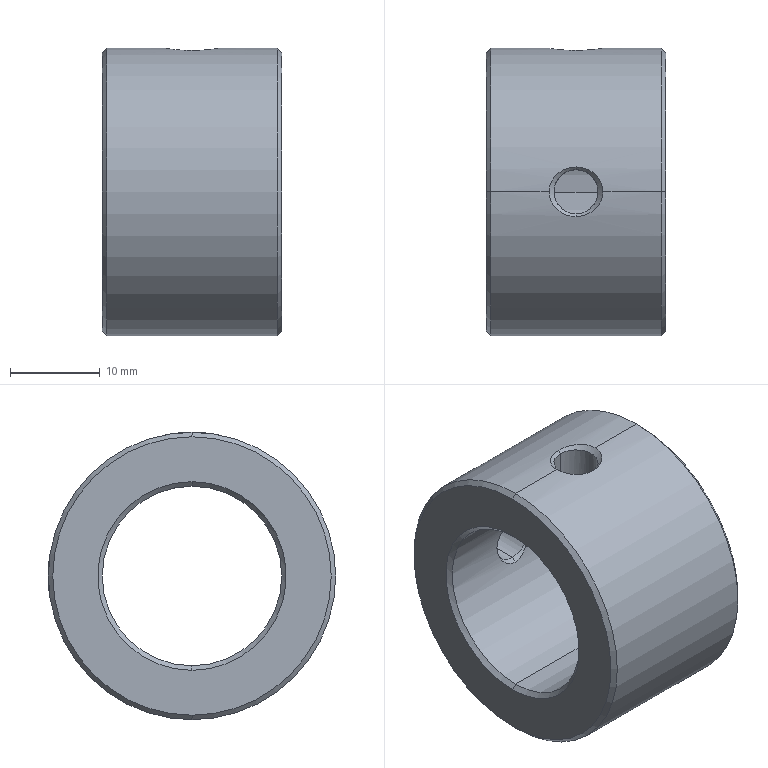Part | STEP file | SCCN20_20 | 1 solid | 28 faces | box 20 x 32 x 32 mm | volume 9528 mm3 | cone 18 | cylinder 8 | plane 2 | commonest cylinder face diameters 4.917 x4 20 x2 32 x2
STEP:
#1=CARTESIAN_POINT('',(0.,-2.458,15.459));
#2=VERTEX_POINT('',#1);
#3=CARTESIAN_POINT('',(0.,2.459,15.459));
#4=VERTEX_POINT('',#3);
#5=CARTESIAN_POINT('',(0.,0.,15.459));
#6=DIRECTION('',(0.,0.,-1.));
#7=DIRECTION('',(0.,1.,0.));
#8=AXIS2_PLACEMENT_3D('',#5,#6,#7);
#9=CIRCLE('',#8,2.459);
#10=EDGE_CURVE('',#2,#4,#9,.T.);
#11=ORIENTED_EDGE('',*,*,#10,.F.);
#12=CARTESIAN_POINT('',(0.,-2.458,10.));
#13=VERTEX_POINT('',#12);
#14=CARTESIAN_POINT('',(0.,-2.458,16.));
#15=DIRECTION('',(0.,0.,-1.));
#16=VECTOR('',#15,1000.);
#17=LINE('',#14,#16);
#18=EDGE_CURVE('',#2,#13,#17,.T.);
#19=ORIENTED_EDGE('',*,*,#18,.T.);
#20=CARTESIAN_POINT('',(-2.458,0.,10.));
#21=VERTEX_POINT('',#20);
#22=CARTESIAN_POINT('',(0.,0.,10.));
#23=DIRECTION('',(0.,0.,-1.));
#24=DIRECTION('',(0.,1.,0.));
#25=AXIS2_PLACEMENT_3D('',#22,#23,#24);
#26=CIRCLE('',#25,2.458);
#27=EDGE_CURVE('',#13,#21,#26,.T.);
#28=ORIENTED_EDGE('',*,*,#27,.T.);
#29=CARTESIAN_POINT('',(0.,2.459,10.));
#30=VERTEX_POINT('',#29);
#31=CARTESIAN_POINT('',(0.,0.,10.));
#32=DIRECTION('',(0.,0.,-1.));
#33=DIRECTION('',(0.,1.,0.));
#34=AXIS2_PLACEMENT_3D('',#31,#32,#33);
#35=CIRCLE('',#34,2.458);
#36=EDGE_CURVE('',#21,#30,#35,.T.);
#37=ORIENTED_EDGE('',*,*,#36,.T.);
#38=CARTESIAN_POINT('',(0.,2.459,16.));
#39=DIRECTION('',(0.,0.,-1.));
#40=VECTOR('',#39,1000.);
#41=LINE('',#38,#40);
#42=EDGE_CURVE('',#4,#30,#41,.T.);
#43=ORIENTED_EDGE('',*,*,#42,.F.);
#44=EDGE_LOOP('',(#11,#19,#28,#37,#43));
#45=FACE_OUTER_BOUND('',#44,.T.);
#46=CARTESIAN_POINT('',(0.,0.,16.));
#47=DIRECTION('',(0.,0.,-1.));
#48=DIRECTION('',(0.,1.,0.));
#49=AXIS2_PLACEMENT_3D('',#46,#47,#48);
#50=CYLINDRICAL_SURFACE('',#49,2.458);
#51=ADVANCED_FACE('',(#45),#50,.F.);
#52=ORIENTED_EDGE('',*,*,#10,.T.);
#53=CARTESIAN_POINT('',(0.,2.76,15.76));
#54=VERTEX_POINT('',#53);
#55=CARTESIAN_POINT('',(0.,3.,16.));
#56=DIRECTION('',(0.,0.7071,0.7071));
#57=VECTOR('',#56,1000.);
#58=LINE('',#55,#57);
#59=EDGE_CURVE('',#4,#54,#58,.T.);
#60=ORIENTED_EDGE('',*,*,#59,.T.);
#61=CARTESIAN_POINT('',(-3.,0.,16.));
#62=VERTEX_POINT('',#61);
#63=CARTESIAN_POINT('',(0.,2.76,15.76));
#64=CARTESIAN_POINT('',(-0.1883,2.76,15.76));
#65=CARTESIAN_POINT('',(-0.3793,2.743,15.763));
#66=CARTESIAN_POINT('',(-0.751,2.677,15.774));
#67=CARTESIAN_POINT('',(-0.9323,2.629,15.783));
#68=CARTESIAN_POINT('',(-1.285,2.499,15.804));
#69=CARTESIAN_POINT('',(-1.459,2.417,15.817));
#70=CARTESIAN_POINT('',(-1.782,2.225,15.845));
#71=CARTESIAN_POINT('',(-1.934,2.116,15.86));
#72=CARTESIAN_POINT('',(-2.216,1.867,15.891));
#73=CARTESIAN_POINT('',(-2.346,1.727,15.907));
#74=CARTESIAN_POINT('',(-2.573,1.428,15.937));
#75=CARTESIAN_POINT('',(-2.671,1.268,15.951));
#76=CARTESIAN_POINT('',(-2.832,0.9263,15.974));
#77=CARTESIAN_POINT('',(-2.895,0.7457,15.984));
#78=CARTESIAN_POINT('',(-2.978,0.3795,15.997));
#79=CARTESIAN_POINT('',(-3.,0.1901,16.));
#80=CARTESIAN_POINT('',(-3.,0.,16.));
#81=B_SPLINE_CURVE_WITH_KNOTS('',3,(#63,#64,#65,#66,#67,#68,#69,#70,#71,#72,#73,#74,#75,#76,#77,#78,#79,#80),.UNSPECIFIED.,.F.,.F.,(4,2,2,2,2,2,2,2,4),(0.01127,0.01184,0.0124,0.01297,0.01354,0.0141,0.01467,0.01523,0.0158),.UNSPECIFIED.);
#82=EDGE_CURVE('',#54,#62,#81,.T.);
#83=ORIENTED_EDGE('',*,*,#82,.T.);
#84=CARTESIAN_POINT('',(0.,-2.76,15.76));
#85=VERTEX_POINT('',#84);
#86=CARTESIAN_POINT('',(-3.,0.,16.));
#87=CARTESIAN_POINT('',(-3.,-0.1897,16.));
#88=CARTESIAN_POINT('',(-2.979,-0.3764,15.997));
#89=CARTESIAN_POINT('',(-2.896,-0.7442,15.984));
#90=CARTESIAN_POINT('',(-2.833,-0.9254,15.974));
#91=CARTESIAN_POINT('',(-2.672,-1.265,15.951));
#92=CARTESIAN_POINT('',(-2.574,-1.427,15.937));
#93=CARTESIAN_POINT('',(-2.345,-1.729,15.907));
#94=CARTESIAN_POINT('',(-2.216,-1.866,15.891));
#95=CARTESIAN_POINT('',(-1.932,-2.117,15.86));
#96=CARTESIAN_POINT('',(-1.779,-2.227,15.845));
#97=CARTESIAN_POINT('',(-1.456,-2.418,15.816));
#98=CARTESIAN_POINT('',(-1.283,-2.5,15.804));
#99=CARTESIAN_POINT('',(-0.9301,-2.629,15.783));
#100=CARTESIAN_POINT('',(-0.7491,-2.678,15.774));
#101=CARTESIAN_POINT('',(-0.3782,-2.744,15.763));
#102=CARTESIAN_POINT('',(-0.1877,-2.76,15.76));
#103=CARTESIAN_POINT('',(0.,-2.76,15.76));
#104=B_SPLINE_CURVE_WITH_KNOTS('',3,(#86,#87,#88,#89,#90,#91,#92,#93,#94,#95,#96,#97,#98,#99,#100,#101,#102,#103),.UNSPECIFIED.,.F.,.F.,(4,2,2,2,2,2,2,2,4),(0.0158,0.01637,0.01693,0.0175,0.01806,0.01862,0.01919,0.01975,0.02032),.UNSPECIFIED.);
#105=EDGE_CURVE('',#62,#85,#104,.T.);
#106=ORIENTED_EDGE('',*,*,#105,.T.);
#107=CARTESIAN_POINT('',(0.,-3.,16.));
#108=DIRECTION('',(0.,-0.7071,0.7071));
#109=VECTOR('',#108,1000.);
#110=LINE('',#107,#109);
#111=EDGE_CURVE('',#2,#85,#110,.T.);
#112=ORIENTED_EDGE('',*,*,#111,.F.);
#113=EDGE_LOOP('',(#52,#60,#83,#106,#112));
#114=FACE_OUTER_BOUND('',#113,.T.);
#115=CARTESIAN_POINT('',(0.,0.,16.));
#116=DIRECTION('',(0.,0.,1.));
#117=DIRECTION('',(0.,-1.,0.));
#118=AXIS2_PLACEMENT_3D('',#115,#116,#117);
#119=CONICAL_SURFACE('',#118,3.,0.7854);
#120=ADVANCED_FACE('',(#114),#119,.F.);
#121=CARTESIAN_POINT('',(2.458,0.,10.));
#122=VERTEX_POINT('',#121);
#123=CARTESIAN_POINT('',(0.,0.,10.));
#124=DIRECTION('',(0.,0.,-1.));
#125=DIRECTION('',(0.,1.,0.));
#126=AXIS2_PLACEMENT_3D('',#123,#124,#125);
#127=CIRCLE('',#126,2.458);
#128=EDGE_CURVE('',#30,#122,#127,.T.);
#129=ORIENTED_EDGE('',*,*,#128,.F.);
#130=CARTESIAN_POINT('',(0.,2.883,9.575));
#131=VERTEX_POINT('',#130);
#132=CARTESIAN_POINT('',(0.,2.459,10.));
#133=DIRECTION('',(0.,0.7071,-0.7071));
#134=VECTOR('',#133,1000.);
#135=LINE('',#132,#134);
#136=EDGE_CURVE('',#30,#131,#135,.T.);
#137=ORIENTED_EDGE('',*,*,#136,.T.);
#138=CARTESIAN_POINT('',(0.,2.883,9.575));
#139=CARTESIAN_POINT('',(0.1747,2.883,9.575));
#140=CARTESIAN_POINT('',(0.3527,2.86,9.583));
#141=CARTESIAN_POINT('',(0.691,2.77,9.609));
#142=CARTESIAN_POINT('',(0.855,2.704,9.628));
#143=CARTESIAN_POINT('',(1.316,2.454,9.696));
#144=CARTESIAN_POINT('',(1.582,2.219,9.755));
#145=CARTESIAN_POINT('',(1.905,1.812,9.836));
#146=CARTESIAN_POINT('',(2.001,1.664,9.862));
#147=CARTESIAN_POINT('',(2.165,1.357,9.909));
#148=CARTESIAN_POINT('',(2.234,1.198,9.929));
#149=CARTESIAN_POINT('',(2.346,0.867,9.964));
#150=CARTESIAN_POINT('',(2.388,0.6945,9.977));
#151=CARTESIAN_POINT('',(2.444,0.3492,9.995));
#152=CARTESIAN_POINT('',(2.459,0.1752,10.));
#153=CARTESIAN_POINT('',(2.458,0.,10.));
#154=B_SPLINE_CURVE_WITH_KNOTS('',3,(#138,#139,#140,#141,#142,#143,#144,#145,#146,#147,#148,#149,#150,#151,#152,#153),.UNSPECIFIED.,.F.,.F.,(4,2,2,2,2,2,2,4),(0.006307,0.00683,0.007353,0.008399,0.008922,0.009445,0.009968,0.01049),.UNSPECIFIED.);
#155=EDGE_CURVE('',#131,#122,#154,.T.);
#156=ORIENTED_EDGE('',*,*,#155,.T.);
#157=EDGE_LOOP('',(#129,#137,#156));
#158=FACE_OUTER_BOUND('',#157,.T.);
#159=CARTESIAN_POINT('',(0.,0.,10.));
#160=DIRECTION('',(0.,0.,-1.));
#161=DIRECTION('',(0.,1.,0.));
#162=AXIS2_PLACEMENT_3D('',#159,#160,#161);
#163=CONICAL_SURFACE('',#162,2.458,0.7854);
#164=ADVANCED_FACE('',(#158),#163,.F.);
#165=CARTESIAN_POINT('',(0.,15.459,2.458));
#166=VERTEX_POINT('',#165);
#167=CARTESIAN_POINT('',(0.,15.459,-2.459));
#168=VERTEX_POINT('',#167);
#169=CARTESIAN_POINT('',(0.,15.459,0.));
#170=DIRECTION('',(0.,-1.,0.));
#171=DIRECTION('',(0.,0.,-1.));
#172=AXIS2_PLACEMENT_3D('',#169,#170,#171);
#173=CIRCLE('',#172,2.458);
#174=EDGE_CURVE('',#166,#168,#173,.T.);
#175=ORIENTED_EDGE('',*,*,#174,.F.);
#176=CARTESIAN_POINT('',(0.,10.,2.458));
#177=VERTEX_POINT('',#176);
#178=CARTESIAN_POINT('',(0.,16.,2.458));
#179=DIRECTION('',(0.,-1.,0.));
#180=VECTOR('',#179,1000.);
#181=LINE('',#178,#180);
#182=EDGE_CURVE('',#166,#177,#181,.T.);
#183=ORIENTED_EDGE('',*,*,#182,.T.);
#184=CARTESIAN_POINT('',(-2.458,10.,0.));
#185=VERTEX_POINT('',#184);
#186=CARTESIAN_POINT('',(0.,10.,0.));
#187=DIRECTION('',(0.,-1.,0.));
#188=DIRECTION('',(0.,0.,-1.));
#189=AXIS2_PLACEMENT_3D('',#186,#187,#188);
#190=CIRCLE('',#189,2.458);
#191=EDGE_CURVE('',#177,#185,#190,.T.);
#192=ORIENTED_EDGE('',*,*,#191,.T.);
#193=CARTESIAN_POINT('',(0.,10.,-2.459));
#194=VERTEX_POINT('',#193);
#195=CARTESIAN_POINT('',(0.,10.,0.));
#196=DIRECTION('',(0.,-1.,0.));
#197=DIRECTION('',(0.,0.,-1.));
#198=AXIS2_PLACEMENT_3D('',#195,#196,#197);
#199=CIRCLE('',#198,2.458);
#200=EDGE_CURVE('',#185,#194,#199,.T.);
#201=ORIENTED_EDGE('',*,*,#200,.T.);
#202=CARTESIAN_POINT('',(0.,16.,-2.459));
#203=DIRECTION('',(0.,-1.,0.));
#204=VECTOR('',#203,1000.);
#205=LINE('',#202,#204);
#206=EDGE_CURVE('',#168,#194,#205,.T.);
#207=ORIENTED_EDGE('',*,*,#206,.F.);
#208=EDGE_LOOP('',(#175,#183,#192,#201,#207));
#209=FACE_OUTER_BOUND('',#208,.T.);
#210=CARTESIAN_POINT('',(0.,16.,0.));
#211=DIRECTION('',(0.,-1.,0.));
#212=DIRECTION('',(0.,0.,-1.));
#213=AXIS2_PLACEMENT_3D('',#210,#211,#212);
#214=CYLINDRICAL_SURFACE('',#213,2.458);
#215=ADVANCED_FACE('',(#209),#214,.F.);
#216=ORIENTED_EDGE('',*,*,#174,.T.);
#217=CARTESIAN_POINT('',(0.,15.76,-2.76));
#218=VERTEX_POINT('',#217);
#219=CARTESIAN_POINT('',(0.,16.,-3.));
#220=DIRECTION('',(0.,0.7071,-0.7071));
#221=VECTOR('',#220,1000.);
#222=LINE('',#219,#221);
#223=EDGE_CURVE('',#168,#218,#222,.T.);
#224=ORIENTED_EDGE('',*,*,#223,.T.);
#225=CARTESIAN_POINT('',(0.,15.76,2.76));
#226=VERTEX_POINT('',#225);
#227=CARTESIAN_POINT('',(0.,15.76,-2.76));
#228=CARTESIAN_POINT('',(-0.1888,15.76,-2.76));
#229=CARTESIAN_POINT('',(-0.3797,15.763,-2.743));
#230=CARTESIAN_POINT('',(-0.7498,15.774,-2.678));
#231=CARTESIAN_POINT('',(-0.9311,15.783,-2.629));
#232=CARTESIAN_POINT('',(-1.286,15.804,-2.499));
#233=CARTESIAN_POINT('',(-1.458,15.817,-2.417));
#234=CARTESIAN_POINT('',(-1.781,15.845,-2.226));
#235=CARTESIAN_POINT('',(-1.935,15.86,-2.115));
#236=CARTESIAN_POINT('',(-2.218,15.892,-1.864));
#237=CARTESIAN_POINT('',(-2.346,15.907,-1.727));
#238=CARTESIAN_POINT('',(-2.574,15.937,-1.427));
#239=CARTESIAN_POINT('',(-2.673,15.951,-1.263));
#240=CARTESIAN_POINT('',(-2.833,15.974,-0.9243));
#241=CARTESIAN_POINT('',(-2.895,15.984,-0.7473));
#242=CARTESIAN_POINT('',(-2.979,15.997,-0.3774));
#243=CARTESIAN_POINT('',(-3.,16.,-0.1885));
#244=CARTESIAN_POINT('',(-3.,16.,0.1871));
#245=CARTESIAN_POINT('',(-2.979,15.997,0.3778));
#246=CARTESIAN_POINT('',(-2.895,15.984,0.7461));
#247=CARTESIAN_POINT('',(-2.833,15.974,0.9237));
#248=CARTESIAN_POINT('',(-2.672,15.951,1.266));
#249=CARTESIAN_POINT('',(-2.573,15.937,1.428));
#250=CARTESIAN_POINT('',(-2.346,15.907,1.727));
#251=CARTESIAN_POINT('',(-2.216,15.891,1.867));
#252=CARTESIAN_POINT('',(-1.933,15.86,2.116));
#253=CARTESIAN_POINT('',(-1.781,15.845,2.226));
#254=CARTESIAN_POINT('',(-1.457,15.817,2.418));
#255=CARTESIAN_POINT('',(-1.284,15.804,2.499));
#256=CARTESIAN_POINT('',(-0.9317,15.783,2.629));
#257=CARTESIAN_POINT('',(-0.7503,15.774,2.678));
#258=CARTESIAN_POINT('',(-0.377,15.763,2.744));
#259=CARTESIAN_POINT('',(-0.1877,15.76,2.76));
#260=CARTESIAN_POINT('',(0.,15.76,2.76));
#261=B_SPLINE_CURVE_WITH_KNOTS('',3,(#227,#228,#229,#230,#231,#232,#233,#234,#235,#236,#237,#238,#239,#240,#241,#242,#243,#244,#245,#246,#247,#248,#249,#250,#251,#252,#253,#254,#255,#256,#257,#258,#259,#260),.UNSPECIFIED.,.F.,.F.,(4,2,2,2,2,2,2,2,2,2,2,2,2,2,2,2,4),(0.01587,0.01644,0.017,0.01757,0.01813,0.0187,0.01926,0.01983,0.02039,0.02096,0.02152,0.02209,0.02265,0.02322,0.02378,0.02435,0.02491),.UNSPECIFIED.);
#262=EDGE_CURVE('',#218,#226,#261,.T.);
#263=ORIENTED_EDGE('',*,*,#262,.T.);
#264=CARTESIAN_POINT('',(0.,16.,3.));
#265=DIRECTION('',(0.,0.7071,0.7071));
#266=VECTOR('',#265,1000.);
#267=LINE('',#264,#266);
#268=EDGE_CURVE('',#166,#226,#267,.T.);
#269=ORIENTED_EDGE('',*,*,#268,.F.);
#270=EDGE_LOOP('',(#216,#224,#263,#269));
#271=FACE_OUTER_BOUND('',#270,.T.);
#272=CARTESIAN_POINT('',(0.,16.,0.));
#273=DIRECTION('',(0.,1.,0.));
#274=DIRECTION('',(0.,0.,1.));
#275=AXIS2_PLACEMENT_3D('',#272,#273,#274);
#276=CONICAL_SURFACE('',#275,3.,0.7854);
#277=ADVANCED_FACE('',(#271),#276,.F.);
#278=CARTESIAN_POINT('',(2.458,10.,0.));
#279=VERTEX_POINT('',#278);
#280=CARTESIAN_POINT('',(0.,10.,0.));
#281=DIRECTION('',(0.,-1.,0.));
#282=DIRECTION('',(0.,0.,-1.));
#283=AXIS2_PLACEMENT_3D('',#280,#281,#282);
#284=CIRCLE('',#283,2.458);
#285=EDGE_CURVE('',#194,#279,#284,.T.);
#286=ORIENTED_EDGE('',*,*,#285,.F.);
#287=CARTESIAN_POINT('',(0.,9.575,-2.883));
#288=VERTEX_POINT('',#287);
#289=CARTESIAN_POINT('',(0.,10.,-2.459));
#290=DIRECTION('',(0.,-0.7071,-0.7071));
#291=VECTOR('',#290,1000.);
#292=LINE('',#289,#291);
#293=EDGE_CURVE('',#194,#288,#292,.T.);
#294=ORIENTED_EDGE('',*,*,#293,.T.);
#295=CARTESIAN_POINT('',(0.,9.575,-2.883));
#296=CARTESIAN_POINT('',(0.1752,9.575,-2.883));
#297=CARTESIAN_POINT('',(0.3529,9.583,-2.86));
#298=CARTESIAN_POINT('',(0.6907,9.609,-2.77));
#299=CARTESIAN_POINT('',(0.8557,9.628,-2.704));
#300=CARTESIAN_POINT('',(1.315,9.696,-2.454));
#301=CARTESIAN_POINT('',(1.582,9.754,-2.22));
#302=CARTESIAN_POINT('',(1.905,9.836,-1.811));
#303=CARTESIAN_POINT('',(2.001,9.862,-1.664));
#304=CARTESIAN_POINT('',(2.165,9.909,-1.358));
#305=CARTESIAN_POINT('',(2.234,9.929,-1.198));
#306=CARTESIAN_POINT('',(2.346,9.964,-0.8661));
#307=CARTESIAN_POINT('',(2.388,9.977,-0.6947));
#308=CARTESIAN_POINT('',(2.444,9.995,-0.3503));
#309=CARTESIAN_POINT('',(2.459,10.,-0.1762));
#310=CARTESIAN_POINT('',(2.458,10.,0.));
#311=B_SPLINE_CURVE_WITH_KNOTS('',3,(#295,#296,#297,#298,#299,#300,#301,#302,#303,#304,#305,#306,#307,#308,#309,#310),.UNSPECIFIED.,.F.,.F.,(4,2,2,2,2,2,2,4),(0.002095,0.00262,0.003146,0.004197,0.004723,0.005249,0.005774,0.0063),.UNSPECIFIED.);
#312=EDGE_CURVE('',#288,#279,#311,.T.);
#313=ORIENTED_EDGE('',*,*,#312,.T.);
#314=EDGE_LOOP('',(#286,#294,#313));
#315=FACE_OUTER_BOUND('',#314,.T.);
#316=CARTESIAN_POINT('',(0.,10.,0.));
#317=DIRECTION('',(0.,-1.,0.));
#318=DIRECTION('',(0.,0.,-1.));
#319=AXIS2_PLACEMENT_3D('',#316,#317,#318);
#320=CONICAL_SURFACE('',#319,2.458,0.7854);
#321=ADVANCED_FACE('',(#315),#320,.F.);
#322=CARTESIAN_POINT('',(-10.,0.,15.5));
#323=VERTEX_POINT('',#322);
#324=CARTESIAN_POINT('',(-10.,0.,-15.5));
#325=VERTEX_POINT('',#324);
#326=CARTESIAN_POINT('',(-10.,0.,0.));
#327=DIRECTION('',(-1.,0.,0.));
#328=DIRECTION('',(0.,0.,1.));
#329=AXIS2_PLACEMENT_3D('',#326,#327,#328);
#330=CIRCLE('',#329,15.5);
#331=EDGE_CURVE('',#323,#325,#330,.T.);
#332=ORIENTED_EDGE('',*,*,#331,.F.);
#333=CARTESIAN_POINT('',(-9.5,0.,16.));
#334=VERTEX_POINT('',#333);
#335=CARTESIAN_POINT('',(-9.5,0.,16.));
#336=DIRECTION('',(0.7071,0.,0.7071));
#337=VECTOR('',#336,1000.);
#338=LINE('',#335,#337);
#339=EDGE_CURVE('',#323,#334,#338,.T.);
#340=ORIENTED_EDGE('',*,*,#339,.T.);
#341=CARTESIAN_POINT('',(-9.5,0.,-16.));
#342=VERTEX_POINT('',#341);
#343=CARTESIAN_POINT('',(-9.5,0.,0.));
#344=DIRECTION('',(-1.,0.,0.));
#345=DIRECTION('',(0.,0.,1.));
#346=AXIS2_PLACEMENT_3D('',#343,#344,#345);
#347=CIRCLE('',#346,16.);
#348=EDGE_CURVE('',#334,#342,#347,.T.);
#349=ORIENTED_EDGE('',*,*,#348,.T.);
#350=CARTESIAN_POINT('',(-9.5,0.,-16.));
#351=DIRECTION('',(0.7071,0.,-0.7071));
#352=VECTOR('',#351,1000.);
#353=LINE('',#350,#352);
#354=EDGE_CURVE('',#325,#342,#353,.T.);
#355=ORIENTED_EDGE('',*,*,#354,.F.);
#356=EDGE_LOOP('',(#332,#340,#349,#355));
#357=FACE_OUTER_BOUND('',#356,.T.);
#358=CARTESIAN_POINT('',(-9.5,0.,0.));
#359=DIRECTION('',(1.,0.,0.));
#360=DIRECTION('',(0.,0.,-1.));
#361=AXIS2_PLACEMENT_3D('',#358,#359,#360);
#362=CONICAL_SURFACE('',#361,16.,0.7854);
#363=ADVANCED_FACE('',(#357),#362,.T.);
#364=CARTESIAN_POINT('',(10.,0.,15.5));
#365=VERTEX_POINT('',#364);
#366=CARTESIAN_POINT('',(10.,0.,-15.5));
#367=VERTEX_POINT('',#366);
#368=CARTESIAN_POINT('',(10.,0.,0.));
#369=DIRECTION('',(-1.,0.,0.));
#370=DIRECTION('',(0.,0.,1.));
#371=AXIS2_PLACEMENT_3D('',#368,#369,#370);
#372=CIRCLE('',#371,15.5);
#373=EDGE_CURVE('',#365,#367,#372,.T.);
#374=ORIENTED_EDGE('',*,*,#373,.T.);
#375=CARTESIAN_POINT('',(9.5,0.,-16.));
#376=VERTEX_POINT('',#375);
#377=CARTESIAN_POINT('',(10.,0.,-15.5));
#378=DIRECTION('',(-0.7071,0.,-0.7071));
#379=VECTOR('',#378,1000.);
#380=LINE('',#377,#379);
#381=EDGE_CURVE('',#367,#376,#380,.T.);
#382=ORIENTED_EDGE('',*,*,#381,.T.);
#383=CARTESIAN_POINT('',(9.5,0.,16.));
#384=VERTEX_POINT('',#383);
#385=CARTESIAN_POINT('',(9.5,0.,0.));
#386=DIRECTION('',(-1.,0.,0.));
#387=DIRECTION('',(0.,0.,1.));
#388=AXIS2_PLACEMENT_3D('',#385,#386,#387);
#389=CIRCLE('',#388,16.);
#390=EDGE_CURVE('',#384,#376,#389,.T.);
#391=ORIENTED_EDGE('',*,*,#390,.F.);
#392=CARTESIAN_POINT('',(10.,0.,15.5));
#393=DIRECTION('',(-0.7071,0.,0.7071));
#394=VECTOR('',#393,1000.);
#395=LINE('',#392,#394);
#396=EDGE_CURVE('',#365,#384,#395,.T.);
#397=ORIENTED_EDGE('',*,*,#396,.F.);
#398=EDGE_LOOP('',(#374,#382,#391,#397));
#399=FACE_OUTER_BOUND('',#398,.T.);
#400=CARTESIAN_POINT('',(10.,0.,0.));
#401=DIRECTION('',(-1.,0.,0.));
#402=DIRECTION('',(0.,0.,1.));
#403=AXIS2_PLACEMENT_3D('',#400,#401,#402);
#404=CONICAL_SURFACE('',#403,15.5,0.7854);
#405=ADVANCED_FACE('',(#399),#404,.T.);
#406=CARTESIAN_POINT('',(9.5,0.,-10.));
#407=VERTEX_POINT('',#406);
#408=CARTESIAN_POINT('',(9.5,0.,10.));
#409=VERTEX_POINT('',#408);
#410=CARTESIAN_POINT('',(9.5,0.,0.));
#411=DIRECTION('',(-1.,0.,0.));
#412=DIRECTION('',(0.,0.,1.));
#413=AXIS2_PLACEMENT_3D('',#410,#411,#412);
#414=CIRCLE('',#413,10.);
#415=EDGE_CURVE('',#407,#409,#414,.T.);
#416=ORIENTED_EDGE('',*,*,#415,.T.);
#417=CARTESIAN_POINT('',(10.,0.,10.5));
#418=VERTEX_POINT('',#417);
#419=CARTESIAN_POINT('',(9.5,0.,10.));
#420=DIRECTION('',(0.7071,0.,0.7071));
#421=VECTOR('',#420,1000.);
#422=LINE('',#419,#421);
#423=EDGE_CURVE('',#409,#418,#422,.T.);
#424=ORIENTED_EDGE('',*,*,#423,.T.);
#425=CARTESIAN_POINT('',(10.,0.,-10.5));
#426=VERTEX_POINT('',#425);
#427=CARTESIAN_POINT('',(10.,0.,0.));
#428=DIRECTION('',(-1.,0.,0.));
#429=DIRECTION('',(0.,0.,1.));
#430=AXIS2_PLACEMENT_3D('',#427,#428,#429);
#431=CIRCLE('',#430,10.5);
#432=EDGE_CURVE('',#426,#418,#431,.T.);
#433=ORIENTED_EDGE('',*,*,#432,.F.);
#434=CARTESIAN_POINT('',(9.5,0.,-10.));
#435=DIRECTION('',(0.7071,0.,-0.7071));
#436=VECTOR('',#435,1000.);
#437=LINE('',#434,#436);
#438=EDGE_CURVE('',#407,#426,#437,.T.);
#439=ORIENTED_EDGE('',*,*,#438,.F.);
#440=EDGE_LOOP('',(#416,#424,#433,#439));
#441=FACE_OUTER_BOUND('',#440,.T.);
#442=CARTESIAN_POINT('',(9.5,0.,0.));
#443=DIRECTION('',(1.,0.,0.));
#444=DIRECTION('',(0.,0.,-1.));
#445=AXIS2_PLACEMENT_3D('',#442,#443,#444);
#446=CONICAL_SURFACE('',#445,10.,0.7854);
#447=ADVANCED_FACE('',(#441),#446,.F.);
#448=CARTESIAN_POINT('',(-9.5,0.,-10.));
#449=VERTEX_POINT('',#448);
#450=CARTESIAN_POINT('',(-9.5,0.,10.));
#451=VERTEX_POINT('',#450);
#452=CARTESIAN_POINT('',(-9.5,0.,0.));
#453=DIRECTION('',(-1.,0.,0.));
#454=DIRECTION('',(0.,0.,1.));
#455=AXIS2_PLACEMENT_3D('',#452,#453,#454);
#456=CIRCLE('',#455,10.);
#457=EDGE_CURVE('',#449,#451,#456,.T.);
#458=ORIENTED_EDGE('',*,*,#457,.F.);
#459=CARTESIAN_POINT('',(-10.,0.,-10.5));
#460=VERTEX_POINT('',#459);
#461=CARTESIAN_POINT('',(-10.,0.,-10.5));
#462=DIRECTION('',(-0.7071,0.,-0.7071));
#463=VECTOR('',#462,1000.);
#464=LINE('',#461,#463);
#465=EDGE_CURVE('',#449,#460,#464,.T.);
#466=ORIENTED_EDGE('',*,*,#465,.T.);
#467=CARTESIAN_POINT('',(-10.,0.,10.5));
#468=VERTEX_POINT('',#467);
#469=CARTESIAN_POINT('',(-10.,0.,0.));
#470=DIRECTION('',(-1.,0.,0.));
#471=DIRECTION('',(0.,0.,1.));
#472=AXIS2_PLACEMENT_3D('',#469,#470,#471);
#473=CIRCLE('',#472,10.5);
#474=EDGE_CURVE('',#460,#468,#473,.T.);
#475=ORIENTED_EDGE('',*,*,#474,.T.);
#476=CARTESIAN_POINT('',(-10.,0.,10.5));
#477=DIRECTION('',(-0.7071,0.,0.7071));
#478=VECTOR('',#477,1000.);
#479=LINE('',#476,#478);
#480=EDGE_CURVE('',#451,#468,#479,.T.);
#481=ORIENTED_EDGE('',*,*,#480,.F.);
#482=EDGE_LOOP('',(#458,#466,#475,#481));
#483=FACE_OUTER_BOUND('',#482,.T.);
#484=CARTESIAN_POINT('',(-10.,0.,0.));
#485=DIRECTION('',(-1.,0.,0.));
#486=DIRECTION('',(0.,0.,1.));
#487=AXIS2_PLACEMENT_3D('',#484,#485,#486);
#488=CONICAL_SURFACE('',#487,10.5,0.7854);
#489=ADVANCED_FACE('',(#483),#488,.F.);
#490=CARTESIAN_POINT('',(0.,15.76,2.76));
#491=CARTESIAN_POINT('',(0.3757,15.76,2.76));
#492=CARTESIAN_POINT('',(0.7561,15.772,2.693));
#493=CARTESIAN_POINT('',(1.46,15.814,2.435));
#494=CARTESIAN_POINT('',(1.793,15.844,2.24));
#495=CARTESIAN_POINT('',(2.213,15.891,1.869));
#496=CARTESIAN_POINT('',(2.344,15.907,1.73));
#497=CARTESIAN_POINT('',(2.572,15.937,1.43));
#498=CARTESIAN_POINT('',(2.67,15.95,1.27));
#499=CARTESIAN_POINT('',(2.831,15.974,0.9309));
#500=CARTESIAN_POINT('',(2.894,15.984,0.7492));
#501=CARTESIAN_POINT('',(2.978,15.996,0.382));
#502=CARTESIAN_POINT('',(3.,16.,0.1953));
#503=CARTESIAN_POINT('',(3.,16.,-0.1841));
#504=CARTESIAN_POINT('',(2.979,15.997,-0.374));
#505=CARTESIAN_POINT('',(2.896,15.984,-0.7411));
#506=CARTESIAN_POINT('',(2.834,15.974,-0.9225));
#507=CARTESIAN_POINT('',(2.673,15.951,-1.264));
#508=CARTESIAN_POINT('',(2.575,15.937,-1.425));
#509=CARTESIAN_POINT('',(2.347,15.907,-1.726));
#510=CARTESIAN_POINT('',(2.217,15.891,-1.865));
#511=CARTESIAN_POINT('',(1.936,15.86,-2.114));
#512=CARTESIAN_POINT('',(1.781,15.845,-2.226));
#513=CARTESIAN_POINT('',(1.456,15.816,-2.418));
#514=CARTESIAN_POINT('',(1.286,15.804,-2.499));
#515=CARTESIAN_POINT('',(0.9327,15.783,-2.629));
#516=CARTESIAN_POINT('',(0.7475,15.774,-2.678));
#517=CARTESIAN_POINT('',(0.3762,15.763,-2.744));
#518=CARTESIAN_POINT('',(0.1889,15.76,-2.76));
#519=CARTESIAN_POINT('',(0.,15.76,-2.76));
#520=B_SPLINE_CURVE_WITH_KNOTS('',3,(#490,#491,#492,#493,#494,#495,#496,#497,#498,#499,#500,#501,#502,#503,#504,#505,#506,#507,#508,#509,#510,#511,#512,#513,#514,#515,#516,#517,#518,#519),.UNSPECIFIED.,.F.,.F.,(4,2,2,2,2,2,2,2,2,2,2,2,2,2,4),(0.006826,0.007957,0.009088,0.009653,0.01022,0.01078,0.01135,0.01191,0.01248,0.01305,0.01361,0.01418,0.01474,0.01531,0.01587),.UNSPECIFIED.);
#521=EDGE_CURVE('',#226,#218,#520,.T.);
#522=ORIENTED_EDGE('',*,*,#521,.F.);
#523=ORIENTED_EDGE('',*,*,#262,.F.);
#524=EDGE_LOOP('',(#522,#523));
#525=FACE_BOUND('',#524,.T.);
#526=ORIENTED_EDGE('',*,*,#390,.T.);
#527=CARTESIAN_POINT('',(5.,0.,-16.));
#528=DIRECTION('',(-1.,0.,0.));
#529=VECTOR('',#528,1000.);
#530=LINE('',#527,#529);
#531=EDGE_CURVE('',#376,#342,#530,.T.);
#532=ORIENTED_EDGE('',*,*,#531,.T.);
#533=ORIENTED_EDGE('',*,*,#348,.F.);
#534=CARTESIAN_POINT('',(5.,0.,16.));
#535=DIRECTION('',(-1.,0.,0.));
#536=VECTOR('',#535,1000.);
#537=LINE('',#534,#536);
#538=EDGE_CURVE('',#62,#334,#537,.T.);
#539=ORIENTED_EDGE('',*,*,#538,.F.);
#540=ORIENTED_EDGE('',*,*,#82,.F.);
#541=CARTESIAN_POINT('',(3.,0.,16.));
#542=VERTEX_POINT('',#541);
#543=CARTESIAN_POINT('',(3.,0.,16.));
#544=CARTESIAN_POINT('',(3.,0.1885,16.));
#545=CARTESIAN_POINT('',(2.978,0.3795,15.997));
#546=CARTESIAN_POINT('',(2.895,0.7462,15.984));
#547=CARTESIAN_POINT('',(2.833,0.9257,15.974));
#548=CARTESIAN_POINT('',(2.671,1.268,15.951));
#549=CARTESIAN_POINT('',(2.573,1.428,15.937));
#550=CARTESIAN_POINT('',(2.345,1.728,15.907));
#551=CARTESIAN_POINT('',(2.215,1.868,15.891));
#552=CARTESIAN_POINT('',(1.792,2.24,15.844));
#553=CARTESIAN_POINT('',(1.46,2.435,15.814));
#554=CARTESIAN_POINT('',(0.9316,2.629,15.783));
#555=CARTESIAN_POINT('',(0.7476,2.678,15.774));
#556=CARTESIAN_POINT('',(0.3751,2.744,15.763));
#557=CARTESIAN_POINT('',(0.188,2.76,15.76));
#558=CARTESIAN_POINT('',(0.,2.76,15.76));
#559=B_SPLINE_CURVE_WITH_KNOTS('',3,(#543,#544,#545,#546,#547,#548,#549,#550,#551,#552,#553,#554,#555,#556,#557,#558),.UNSPECIFIED.,.F.,.F.,(4,2,2,2,2,2,2,4),(0.006751,0.007316,0.007881,0.008446,0.009012,0.01014,0.01071,0.01127),.UNSPECIFIED.);
#560=EDGE_CURVE('',#542,#54,#559,.T.);
#561=ORIENTED_EDGE('',*,*,#560,.F.);
#562=CARTESIAN_POINT('',(5.,0.,16.));
#563=DIRECTION('',(-1.,0.,0.));
#564=VECTOR('',#563,1000.);
#565=LINE('',#562,#564);
#566=EDGE_CURVE('',#384,#542,#565,.T.);
#567=ORIENTED_EDGE('',*,*,#566,.F.);
#568=EDGE_LOOP('',(#526,#532,#533,#539,#540,#561,#567));
#569=FACE_OUTER_BOUND('',#568,.T.);
#570=CARTESIAN_POINT('',(5.,0.,0.));
#571=DIRECTION('',(-1.,0.,0.));
#572=DIRECTION('',(0.,0.,1.));
#573=AXIS2_PLACEMENT_3D('',#570,#571,#572);
#574=CYLINDRICAL_SURFACE('',#573,16.);
#575=ADVANCED_FACE('',(#525,#569),#574,.T.);
#576=ORIENTED_EDGE('',*,*,#415,.F.);
#577=CARTESIAN_POINT('',(5.,0.,-10.));
#578=DIRECTION('',(-1.,0.,0.));
#579=VECTOR('',#578,1000.);
#580=LINE('',#577,#579);
#581=EDGE_CURVE('',#407,#449,#580,.T.);
#582=ORIENTED_EDGE('',*,*,#581,.T.);
#583=ORIENTED_EDGE('',*,*,#457,.T.);
#584=CARTESIAN_POINT('',(5.,0.,10.));
#585=DIRECTION('',(-1.,0.,0.));
#586=VECTOR('',#585,1000.);
#587=LINE('',#584,#586);
#588=EDGE_CURVE('',#21,#451,#587,.T.);
#589=ORIENTED_EDGE('',*,*,#588,.F.);
#590=CARTESIAN_POINT('',(2.458,0.,10.));
#591=CARTESIAN_POINT('',(2.459,-0.1753,10.));
#592=CARTESIAN_POINT('',(2.444,-0.353,9.995));
#593=CARTESIAN_POINT('',(2.388,-0.6983,9.977));
#594=CARTESIAN_POINT('',(2.346,-0.8672,9.964));
#595=CARTESIAN_POINT('',(2.234,-1.198,9.929));
#596=CARTESIAN_POINT('',(2.164,-1.361,9.908));
#597=CARTESIAN_POINT('',(2.,-1.666,9.861));
#598=CARTESIAN_POINT('',(1.905,-1.811,9.836));
#599=CARTESIAN_POINT('',(1.69,-2.082,9.782));
#600=CARTESIAN_POINT('',(1.569,-2.21,9.753));
#601=CARTESIAN_POINT('',(1.306,-2.436,9.699));
#602=CARTESIAN_POINT('',(1.165,-2.536,9.674));
#603=CARTESIAN_POINT('',(0.8556,-2.704,9.628));
#604=CARTESIAN_POINT('',(0.6932,-2.769,9.609));
#605=CARTESIAN_POINT('',(0.3544,-2.859,9.583));
#606=CARTESIAN_POINT('',(0.1765,-2.883,9.575));
#607=CARTESIAN_POINT('',(-0.1734,-2.883,9.575));
#608=CARTESIAN_POINT('',(-0.3506,-2.86,9.582));
#609=CARTESIAN_POINT('',(-0.6906,-2.77,9.609));
#610=CARTESIAN_POINT('',(-0.8532,-2.705,9.628));
#611=CARTESIAN_POINT('',(-1.163,-2.537,9.673));
#612=CARTESIAN_POINT('',(-1.305,-2.437,9.699));
#613=CARTESIAN_POINT('',(-1.569,-2.21,9.753));
#614=CARTESIAN_POINT('',(-1.691,-2.082,9.782));
#615=CARTESIAN_POINT('',(-2.015,-1.671,9.863));
#616=CARTESIAN_POINT('',(-2.178,-1.364,9.912));
#617=CARTESIAN_POINT('',(-2.346,-0.8651,9.964));
#618=CARTESIAN_POINT('',(-2.388,-0.6959,9.977));
#619=CARTESIAN_POINT('',(-2.444,-0.352,9.995));
#620=CARTESIAN_POINT('',(-2.459,-0.1762,10.));
#621=CARTESIAN_POINT('',(-2.458,0.,10.));
#622=B_SPLINE_CURVE_WITH_KNOTS('',3,(#590,#591,#592,#593,#594,#595,#596,#597,#598,#599,#600,#601,#602,#603,#604,#605,#606,#607,#608,#609,#610,#611,#612,#613,#614,#615,#616,#617,#618,#619,#620,#621),.UNSPECIFIED.,.F.,.F.,(4,2,2,2,2,2,2,2,2,2,2,2,2,2,2,4),(0.01049,0.01101,0.01154,0.01206,0.01258,0.01311,0.01363,0.01415,0.01468,0.0152,0.01572,0.01625,0.01677,0.01782,0.01834,0.01886),.UNSPECIFIED.);
#623=EDGE_CURVE('',#122,#21,#622,.T.);
#624=ORIENTED_EDGE('',*,*,#623,.F.);
#625=CARTESIAN_POINT('',(5.,0.,10.));
#626=DIRECTION('',(-1.,0.,0.));
#627=VECTOR('',#626,1000.);
#628=LINE('',#625,#627);
#629=EDGE_CURVE('',#409,#122,#628,.T.);
#630=ORIENTED_EDGE('',*,*,#629,.F.);
#631=EDGE_LOOP('',(#576,#582,#583,#589,#624,#630));
#632=FACE_OUTER_BOUND('',#631,.T.);
#633=CARTESIAN_POINT('',(5.,0.,0.));
#634=DIRECTION('',(-1.,0.,0.));
#635=DIRECTION('',(0.,0.,1.));
#636=AXIS2_PLACEMENT_3D('',#633,#634,#635);
#637=CYLINDRICAL_SURFACE('',#636,10.);
#638=ADVANCED_FACE('',(#632),#637,.F.);
#639=ORIENTED_EDGE('',*,*,#581,.F.);
#640=CARTESIAN_POINT('',(9.5,0.,0.));
#641=DIRECTION('',(-1.,0.,0.));
#642=DIRECTION('',(0.,0.,1.));
#643=AXIS2_PLACEMENT_3D('',#640,#641,#642);
#644=CIRCLE('',#643,10.);
#645=EDGE_CURVE('',#409,#407,#644,.T.);
#646=ORIENTED_EDGE('',*,*,#645,.F.);
#647=ORIENTED_EDGE('',*,*,#629,.T.);
#648=ORIENTED_EDGE('',*,*,#155,.F.);
#649=CARTESIAN_POINT('',(-2.458,0.,10.));
#650=CARTESIAN_POINT('',(-2.459,0.1767,10.));
#651=CARTESIAN_POINT('',(-2.444,0.3512,9.995));
#652=CARTESIAN_POINT('',(-2.388,0.696,9.977));
#653=CARTESIAN_POINT('',(-2.346,0.8674,9.964));
#654=CARTESIAN_POINT('',(-2.233,1.201,9.929));
#655=CARTESIAN_POINT('',(-2.164,1.36,9.908));
#656=CARTESIAN_POINT('',(-2.,1.665,9.862));
#657=CARTESIAN_POINT('',(-1.904,1.812,9.835));
#658=CARTESIAN_POINT('',(-1.688,2.086,9.781));
#659=CARTESIAN_POINT('',(-1.569,2.211,9.753));
#660=CARTESIAN_POINT('',(-1.307,2.436,9.7));
#661=CARTESIAN_POINT('',(-1.163,2.537,9.673));
#662=CARTESIAN_POINT('',(-0.855,2.704,9.628));
#663=CARTESIAN_POINT('',(-0.6931,2.77,9.609));
#664=CARTESIAN_POINT('',(-0.3517,2.86,9.582));
#665=CARTESIAN_POINT('',(-0.1754,2.883,9.575));
#666=CARTESIAN_POINT('',(0.,2.883,9.575));
#667=B_SPLINE_CURVE_WITH_KNOTS('',3,(#649,#650,#651,#652,#653,#654,#655,#656,#657,#658,#659,#660,#661,#662,#663,#664,#665,#666),.UNSPECIFIED.,.F.,.F.,(4,2,2,2,2,2,2,2,4),(0.002109,0.002634,0.003158,0.003683,0.004208,0.004733,0.005258,0.005782,0.006307),.UNSPECIFIED.);
#668=EDGE_CURVE('',#21,#131,#667,.T.);
#669=ORIENTED_EDGE('',*,*,#668,.F.);
#670=ORIENTED_EDGE('',*,*,#588,.T.);
#671=CARTESIAN_POINT('',(-9.5,0.,0.));
#672=DIRECTION('',(-1.,0.,0.));
#673=DIRECTION('',(0.,0.,1.));
#674=AXIS2_PLACEMENT_3D('',#671,#672,#673);
#675=CIRCLE('',#674,10.);
#676=EDGE_CURVE('',#451,#449,#675,.T.);
#677=ORIENTED_EDGE('',*,*,#676,.T.);
#678=EDGE_LOOP('',(#639,#646,#647,#648,#669,#670,#677));
#679=FACE_OUTER_BOUND('',#678,.T.);
#680=CARTESIAN_POINT('',(2.458,10.,0.));
#681=CARTESIAN_POINT('',(2.459,10.,0.1762));
#682=CARTESIAN_POINT('',(2.444,9.995,0.3525));
#683=CARTESIAN_POINT('',(2.388,9.977,0.6966));
#684=CARTESIAN_POINT('',(2.346,9.964,0.8658));
#685=CARTESIAN_POINT('',(2.234,9.929,1.198));
#686=CARTESIAN_POINT('',(2.164,9.908,1.359));
#687=CARTESIAN_POINT('',(2.001,9.862,1.664));
#688=CARTESIAN_POINT('',(1.907,9.836,1.809));
#689=CARTESIAN_POINT('',(1.691,9.782,2.082));
#690=CARTESIAN_POINT('',(1.57,9.754,2.209));
#691=CARTESIAN_POINT('',(1.31,9.7,2.433));
#692=CARTESIAN_POINT('',(1.169,9.674,2.533));
#693=CARTESIAN_POINT('',(0.8617,9.629,2.701));
#694=CARTESIAN_POINT('',(0.6984,9.61,2.768));
#695=CARTESIAN_POINT('',(0.3601,9.583,2.858));
#696=CARTESIAN_POINT('',(0.182,9.576,2.883));
#697=CARTESIAN_POINT('',(-0.1682,9.575,2.884));
#698=CARTESIAN_POINT('',(-0.3451,9.582,2.861));
#699=CARTESIAN_POINT('',(-0.6858,9.608,2.772));
#700=CARTESIAN_POINT('',(-0.8481,9.627,2.707));
#701=CARTESIAN_POINT('',(-1.158,9.672,2.54));
#702=CARTESIAN_POINT('',(-1.301,9.698,2.44));
#703=CARTESIAN_POINT('',(-1.566,9.753,2.214));
#704=CARTESIAN_POINT('',(-1.687,9.781,2.086));
#705=CARTESIAN_POINT('',(-2.011,9.862,1.678));
#706=CARTESIAN_POINT('',(-2.178,9.912,1.364));
#707=CARTESIAN_POINT('',(-2.345,9.964,0.8689));
#708=CARTESIAN_POINT('',(-2.388,9.977,0.6975));
#709=CARTESIAN_POINT('',(-2.445,9.995,0.3494));
#710=CARTESIAN_POINT('',(-2.459,10.,0.1749));
#711=CARTESIAN_POINT('',(-2.458,10.,0.));
#712=B_SPLINE_CURVE_WITH_KNOTS('',3,(#680,#681,#682,#683,#684,#685,#686,#687,#688,#689,#690,#691,#692,#693,#694,#695,#696,#697,#698,#699,#700,#701,#702,#703,#704,#705,#706,#707,#708,#709,#710,#711),.UNSPECIFIED.,.F.,.F.,(4,2,2,2,2,2,2,2,2,2,2,2,2,2,2,4),(0.0063,0.006826,0.007351,0.007877,0.008403,0.008928,0.009454,0.00998,0.01051,0.01103,0.01156,0.01208,0.01261,0.01366,0.01418,0.01471),.UNSPECIFIED.);
#713=EDGE_CURVE('',#279,#185,#712,.T.);
#714=ORIENTED_EDGE('',*,*,#713,.F.);
#715=ORIENTED_EDGE('',*,*,#312,.F.);
#716=CARTESIAN_POINT('',(-2.458,10.,0.));
#717=CARTESIAN_POINT('',(-2.459,10.,-0.1749));
#718=CARTESIAN_POINT('',(-2.444,9.995,-0.3515));
#719=CARTESIAN_POINT('',(-2.387,9.977,-0.6993));
#720=CARTESIAN_POINT('',(-2.345,9.964,-0.8687));
#721=CARTESIAN_POINT('',(-2.178,9.912,-1.363));
#722=CARTESIAN_POINT('',(-2.012,9.862,-1.677));
#723=CARTESIAN_POINT('',(-1.685,9.78,-2.089));
#724=CARTESIAN_POINT('',(-1.565,9.753,-2.214));
#725=CARTESIAN_POINT('',(-1.302,9.699,-2.439));
#726=CARTESIAN_POINT('',(-1.157,9.672,-2.54));
#727=CARTESIAN_POINT('',(-0.8517,9.627,-2.705));
#728=CARTESIAN_POINT('',(-0.689,9.609,-2.771));
#729=CARTESIAN_POINT('',(-0.348,9.582,-2.861));
#730=CARTESIAN_POINT('',(-0.1752,9.575,-2.883));
#731=CARTESIAN_POINT('',(0.,9.575,-2.883));
#732=B_SPLINE_CURVE_WITH_KNOTS('',3,(#716,#717,#718,#719,#720,#721,#722,#723,#724,#725,#726,#727,#728,#729,#730,#731),.UNSPECIFIED.,.F.,.F.,(4,2,2,2,2,2,2,4),(0.01471,0.01524,0.01576,0.01681,0.01734,0.01786,0.01839,0.01891),.UNSPECIFIED.);
#733=EDGE_CURVE('',#185,#288,#732,.T.);
#734=ORIENTED_EDGE('',*,*,#733,.F.);
#735=EDGE_LOOP('',(#714,#715,#734));
#736=FACE_BOUND('',#735,.T.);
#737=CARTESIAN_POINT('',(5.,0.,0.));
#738=DIRECTION('',(-1.,0.,0.));
#739=DIRECTION('',(0.,0.,1.));
#740=AXIS2_PLACEMENT_3D('',#737,#738,#739);
#741=CYLINDRICAL_SURFACE('',#740,10.);
#742=ADVANCED_FACE('',(#679,#736),#741,.F.);
#743=ORIENTED_EDGE('',*,*,#531,.F.);
#744=CARTESIAN_POINT('',(9.5,0.,0.));
#745=DIRECTION('',(-1.,0.,0.));
#746=DIRECTION('',(0.,0.,1.));
#747=AXIS2_PLACEMENT_3D('',#744,#745,#746);
#748=CIRCLE('',#747,16.);
#749=EDGE_CURVE('',#376,#384,#748,.T.);
#750=ORIENTED_EDGE('',*,*,#749,.T.);
#751=ORIENTED_EDGE('',*,*,#566,.T.);
#752=CARTESIAN_POINT('',(0.,-2.76,15.76));
#753=CARTESIAN_POINT('',(0.1884,-2.76,15.76));
#754=CARTESIAN_POINT('',(0.3758,-2.744,15.763));
#755=CARTESIAN_POINT('',(0.7487,-2.678,15.774));
#756=CARTESIAN_POINT('',(0.9333,-2.628,15.783));
#757=CARTESIAN_POINT('',(1.286,-2.499,15.804));
#758=CARTESIAN_POINT('',(1.456,-2.419,15.816));
#759=CARTESIAN_POINT('',(1.781,-2.226,15.845));
#760=CARTESIAN_POINT('',(1.935,-2.114,15.86));
#761=CARTESIAN_POINT('',(2.216,-1.866,15.891));
#762=CARTESIAN_POINT('',(2.344,-1.729,15.907));
#763=CARTESIAN_POINT('',(2.574,-1.427,15.937));
#764=CARTESIAN_POINT('',(2.672,-1.266,15.951));
#765=CARTESIAN_POINT('',(2.832,-0.9265,15.974));
#766=CARTESIAN_POINT('',(2.895,-0.7459,15.984));
#767=CARTESIAN_POINT('',(2.979,-0.376,15.997));
#768=CARTESIAN_POINT('',(3.,-0.189,16.));
#769=CARTESIAN_POINT('',(3.,0.,16.));
#770=B_SPLINE_CURVE_WITH_KNOTS('',3,(#752,#753,#754,#755,#756,#757,#758,#759,#760,#761,#762,#763,#764,#765,#766,#767,#768,#769),.UNSPECIFIED.,.F.,.F.,(4,2,2,2,2,2,2,2,4),(0.002216,0.002783,0.00335,0.003917,0.004484,0.00505,0.005617,0.006184,0.006751),.UNSPECIFIED.);
#771=EDGE_CURVE('',#85,#542,#770,.T.);
#772=ORIENTED_EDGE('',*,*,#771,.F.);
#773=ORIENTED_EDGE('',*,*,#105,.F.);
#774=ORIENTED_EDGE('',*,*,#538,.T.);
#775=CARTESIAN_POINT('',(-9.5,0.,0.));
#776=DIRECTION('',(-1.,0.,0.));
#777=DIRECTION('',(0.,0.,1.));
#778=AXIS2_PLACEMENT_3D('',#775,#776,#777);
#779=CIRCLE('',#778,16.);
#780=EDGE_CURVE('',#342,#334,#779,.T.);
#781=ORIENTED_EDGE('',*,*,#780,.F.);
#782=EDGE_LOOP('',(#743,#750,#751,#772,#773,#774,#781));
#783=FACE_OUTER_BOUND('',#782,.T.);
#784=CARTESIAN_POINT('',(5.,0.,0.));
#785=DIRECTION('',(-1.,0.,0.));
#786=DIRECTION('',(0.,0.,1.));
#787=AXIS2_PLACEMENT_3D('',#784,#785,#786);
#788=CYLINDRICAL_SURFACE('',#787,16.);
#789=ADVANCED_FACE('',(#783),#788,.T.);
#790=CARTESIAN_POINT('',(-10.,0.,0.));
#791=DIRECTION('',(-1.,0.,0.));
#792=DIRECTION('',(0.,0.,1.));
#793=AXIS2_PLACEMENT_3D('',#790,#791,#792);
#794=CIRCLE('',#793,10.5);
#795=EDGE_CURVE('',#468,#460,#794,.T.);
#796=ORIENTED_EDGE('',*,*,#795,.F.);
#797=ORIENTED_EDGE('',*,*,#474,.F.);
#798=EDGE_LOOP('',(#796,#797));
#799=FACE_BOUND('',#798,.T.);
#800=CARTESIAN_POINT('',(-10.,0.,0.));
#801=DIRECTION('',(-1.,0.,0.));
#802=DIRECTION('',(0.,0.,1.));
#803=AXIS2_PLACEMENT_3D('',#800,#801,#802);
#804=CIRCLE('',#803,15.5);
#805=EDGE_CURVE('',#325,#323,#804,.T.);
#806=ORIENTED_EDGE('',*,*,#805,.T.);
#807=ORIENTED_EDGE('',*,*,#331,.T.);
#808=EDGE_LOOP('',(#806,#807));
#809=FACE_OUTER_BOUND('',#808,.T.);
#810=CARTESIAN_POINT('',(-10.,15.5,0.));
#811=DIRECTION('',(1.,0.,0.));
#812=DIRECTION('',(0.,0.,-1.));
#813=AXIS2_PLACEMENT_3D('',#810,#811,#812);
#814=PLANE('',#813);
#815=ADVANCED_FACE('',(#799,#809),#814,.F.);
#816=ORIENTED_EDGE('',*,*,#465,.F.);
#817=ORIENTED_EDGE('',*,*,#676,.F.);
#818=ORIENTED_EDGE('',*,*,#480,.T.);
#819=ORIENTED_EDGE('',*,*,#795,.T.);
#820=EDGE_LOOP('',(#816,#817,#818,#819));
#821=FACE_OUTER_BOUND('',#820,.T.);
#822=CARTESIAN_POINT('',(-10.,0.,0.));
#823=DIRECTION('',(-1.,0.,0.));
#824=DIRECTION('',(0.,0.,1.));
#825=AXIS2_PLACEMENT_3D('',#822,#823,#824);
#826=CONICAL_SURFACE('',#825,10.5,0.7854);
#827=ADVANCED_FACE('',(#821),#826,.F.);
#828=ORIENTED_EDGE('',*,*,#423,.F.);
#829=ORIENTED_EDGE('',*,*,#645,.T.);
#830=ORIENTED_EDGE('',*,*,#438,.T.);
#831=CARTESIAN_POINT('',(10.,0.,0.));
#832=DIRECTION('',(-1.,0.,0.));
#833=DIRECTION('',(0.,0.,1.));
#834=AXIS2_PLACEMENT_3D('',#831,#832,#833);
#835=CIRCLE('',#834,10.5);
#836=EDGE_CURVE('',#418,#426,#835,.T.);
#837=ORIENTED_EDGE('',*,*,#836,.F.);
#838=EDGE_LOOP('',(#828,#829,#830,#837));
#839=FACE_OUTER_BOUND('',#838,.T.);
#840=CARTESIAN_POINT('',(9.5,0.,0.));
#841=DIRECTION('',(1.,0.,0.));
#842=DIRECTION('',(0.,0.,-1.));
#843=AXIS2_PLACEMENT_3D('',#840,#841,#842);
#844=CONICAL_SURFACE('',#843,10.,0.7854);
#845=ADVANCED_FACE('',(#839),#844,.F.);
#846=ORIENTED_EDGE('',*,*,#373,.F.);
#847=CARTESIAN_POINT('',(10.,0.,0.));
#848=DIRECTION('',(-1.,0.,0.));
#849=DIRECTION('',(0.,0.,1.));
#850=AXIS2_PLACEMENT_3D('',#847,#848,#849);
#851=CIRCLE('',#850,15.5);
#852=EDGE_CURVE('',#367,#365,#851,.T.);
#853=ORIENTED_EDGE('',*,*,#852,.F.);
#854=EDGE_LOOP('',(#846,#853));
#855=FACE_OUTER_BOUND('',#854,.T.);
#856=ORIENTED_EDGE('',*,*,#432,.T.);
#857=ORIENTED_EDGE('',*,*,#836,.T.);
#858=EDGE_LOOP('',(#856,#857));
#859=FACE_BOUND('',#858,.T.);
#860=CARTESIAN_POINT('',(10.,10.5,0.));
#861=DIRECTION('',(-1.,0.,0.));
#862=DIRECTION('',(0.,0.,1.));
#863=AXIS2_PLACEMENT_3D('',#860,#861,#862);
#864=PLANE('',#863);
#865=ADVANCED_FACE('',(#855,#859),#864,.F.);
#866=ORIENTED_EDGE('',*,*,#381,.F.);
#867=ORIENTED_EDGE('',*,*,#852,.T.);
#868=ORIENTED_EDGE('',*,*,#396,.T.);
#869=ORIENTED_EDGE('',*,*,#749,.F.);
#870=EDGE_LOOP('',(#866,#867,#868,#869));
#871=FACE_OUTER_BOUND('',#870,.T.);
#872=CARTESIAN_POINT('',(10.,0.,0.));
#873=DIRECTION('',(-1.,0.,0.));
#874=DIRECTION('',(0.,0.,1.));
#875=AXIS2_PLACEMENT_3D('',#872,#873,#874);
#876=CONICAL_SURFACE('',#875,15.5,0.7854);
#877=ADVANCED_FACE('',(#871),#876,.T.);
#878=ORIENTED_EDGE('',*,*,#339,.F.);
#879=ORIENTED_EDGE('',*,*,#805,.F.);
#880=ORIENTED_EDGE('',*,*,#354,.T.);
#881=ORIENTED_EDGE('',*,*,#780,.T.);
#882=EDGE_LOOP('',(#878,#879,#880,#881));
#883=FACE_OUTER_BOUND('',#882,.T.);
#884=CARTESIAN_POINT('',(-9.5,0.,0.));
#885=DIRECTION('',(1.,0.,0.));
#886=DIRECTION('',(0.,0.,-1.));
#887=AXIS2_PLACEMENT_3D('',#884,#885,#886);
#888=CONICAL_SURFACE('',#887,16.,0.7854);
#889=ADVANCED_FACE('',(#883),#888,.T.);
#890=ORIENTED_EDGE('',*,*,#713,.T.);
#891=ORIENTED_EDGE('',*,*,#191,.F.);
#892=CARTESIAN_POINT('',(0.,10.,0.));
#893=DIRECTION('',(0.,-1.,0.));
#894=DIRECTION('',(0.,0.,-1.));
#895=AXIS2_PLACEMENT_3D('',#892,#893,#894);
#896=CIRCLE('',#895,2.458);
#897=EDGE_CURVE('',#279,#177,#896,.T.);
#898=ORIENTED_EDGE('',*,*,#897,.F.);
#899=EDGE_LOOP('',(#890,#891,#898));
#900=FACE_OUTER_BOUND('',#899,.T.);
#901=CARTESIAN_POINT('',(0.,10.,0.));
#902=DIRECTION('',(0.,-1.,0.));
#903=DIRECTION('',(0.,0.,-1.));
#904=AXIS2_PLACEMENT_3D('',#901,#902,#903);
#905=CONICAL_SURFACE('',#904,2.458,0.7854);
#906=ADVANCED_FACE('',(#900),#905,.F.);
#907=ORIENTED_EDGE('',*,*,#293,.F.);
#908=ORIENTED_EDGE('',*,*,#200,.F.);
#909=ORIENTED_EDGE('',*,*,#733,.T.);
#910=EDGE_LOOP('',(#907,#908,#909));
#911=FACE_OUTER_BOUND('',#910,.T.);
#912=CARTESIAN_POINT('',(0.,10.,0.));
#913=DIRECTION('',(0.,-1.,0.));
#914=DIRECTION('',(0.,0.,-1.));
#915=AXIS2_PLACEMENT_3D('',#912,#913,#914);
#916=CONICAL_SURFACE('',#915,2.458,0.7854);
#917=ADVANCED_FACE('',(#911),#916,.F.);
#918=ORIENTED_EDGE('',*,*,#223,.F.);
#919=CARTESIAN_POINT('',(0.,15.459,0.));
#920=DIRECTION('',(0.,-1.,0.));
#921=DIRECTION('',(0.,0.,-1.));
#922=AXIS2_PLACEMENT_3D('',#919,#920,#921);
#923=CIRCLE('',#922,2.458);
#924=EDGE_CURVE('',#168,#166,#923,.T.);
#925=ORIENTED_EDGE('',*,*,#924,.T.);
#926=ORIENTED_EDGE('',*,*,#268,.T.);
#927=ORIENTED_EDGE('',*,*,#521,.T.);
#928=EDGE_LOOP('',(#918,#925,#926,#927));
#929=FACE_OUTER_BOUND('',#928,.T.);
#930=CARTESIAN_POINT('',(0.,16.,0.));
#931=DIRECTION('',(0.,1.,0.));
#932=DIRECTION('',(0.,0.,1.));
#933=AXIS2_PLACEMENT_3D('',#930,#931,#932);
#934=CONICAL_SURFACE('',#933,3.,0.7854);
#935=ADVANCED_FACE('',(#929),#934,.F.);
#936=ORIENTED_EDGE('',*,*,#182,.F.);
#937=ORIENTED_EDGE('',*,*,#924,.F.);
#938=ORIENTED_EDGE('',*,*,#206,.T.);
#939=ORIENTED_EDGE('',*,*,#285,.T.);
#940=ORIENTED_EDGE('',*,*,#897,.T.);
#941=EDGE_LOOP('',(#936,#937,#938,#939,#940));
#942=FACE_OUTER_BOUND('',#941,.T.);
#943=CARTESIAN_POINT('',(0.,16.,0.));
#944=DIRECTION('',(0.,-1.,0.));
#945=DIRECTION('',(0.,0.,-1.));
#946=AXIS2_PLACEMENT_3D('',#943,#944,#945);
#947=CYLINDRICAL_SURFACE('',#946,2.458);
#948=ADVANCED_FACE('',(#942),#947,.F.);
#949=ORIENTED_EDGE('',*,*,#136,.F.);
#950=ORIENTED_EDGE('',*,*,#36,.F.);
#951=ORIENTED_EDGE('',*,*,#668,.T.);
#952=EDGE_LOOP('',(#949,#950,#951));
#953=FACE_OUTER_BOUND('',#952,.T.);
#954=CARTESIAN_POINT('',(0.,0.,10.));
#955=DIRECTION('',(0.,0.,-1.));
#956=DIRECTION('',(0.,1.,0.));
#957=AXIS2_PLACEMENT_3D('',#954,#955,#956);
#958=CONICAL_SURFACE('',#957,2.458,0.7854);
#959=ADVANCED_FACE('',(#953),#958,.F.);
#960=ORIENTED_EDGE('',*,*,#623,.T.);
#961=ORIENTED_EDGE('',*,*,#27,.F.);
#962=CARTESIAN_POINT('',(0.,0.,10.));
#963=DIRECTION('',(0.,0.,-1.));
#964=DIRECTION('',(0.,1.,0.));
#965=AXIS2_PLACEMENT_3D('',#962,#963,#964);
#966=CIRCLE('',#965,2.458);
#967=EDGE_CURVE('',#122,#13,#966,.T.);
#968=ORIENTED_EDGE('',*,*,#967,.F.);
#969=EDGE_LOOP('',(#960,#961,#968));
#970=FACE_OUTER_BOUND('',#969,.T.);
#971=CARTESIAN_POINT('',(0.,0.,10.));
#972=DIRECTION('',(0.,0.,-1.));
#973=DIRECTION('',(0.,1.,0.));
#974=AXIS2_PLACEMENT_3D('',#971,#972,#973);
#975=CONICAL_SURFACE('',#974,2.458,0.7854);
#976=ADVANCED_FACE('',(#970),#975,.F.);
#977=ORIENTED_EDGE('',*,*,#59,.F.);
#978=CARTESIAN_POINT('',(0.,0.,15.459));
#979=DIRECTION('',(0.,0.,-1.));
#980=DIRECTION('',(0.,1.,0.));
#981=AXIS2_PLACEMENT_3D('',#978,#979,#980);
#982=CIRCLE('',#981,2.459);
#983=EDGE_CURVE('',#4,#2,#982,.T.);
#984=ORIENTED_EDGE('',*,*,#983,.T.);
#985=ORIENTED_EDGE('',*,*,#111,.T.);
#986=ORIENTED_EDGE('',*,*,#771,.T.);
#987=ORIENTED_EDGE('',*,*,#560,.T.);
#988=EDGE_LOOP('',(#977,#984,#985,#986,#987));
#989=FACE_OUTER_BOUND('',#988,.T.);
#990=CARTESIAN_POINT('',(0.,0.,16.));
#991=DIRECTION('',(0.,0.,1.));
#992=DIRECTION('',(0.,-1.,0.));
#993=AXIS2_PLACEMENT_3D('',#990,#991,#992);
#994=CONICAL_SURFACE('',#993,3.,0.7854);
#995=ADVANCED_FACE('',(#989),#994,.F.);
#996=ORIENTED_EDGE('',*,*,#18,.F.);
#997=ORIENTED_EDGE('',*,*,#983,.F.);
#998=ORIENTED_EDGE('',*,*,#42,.T.);
#999=ORIENTED_EDGE('',*,*,#128,.T.);
#1000=ORIENTED_EDGE('',*,*,#967,.T.);
#1001=EDGE_LOOP('',(#996,#997,#998,#999,#1000));
#1002=FACE_OUTER_BOUND('',#1001,.T.);
#1003=CARTESIAN_POINT('',(0.,0.,16.));
#1004=DIRECTION('',(0.,0.,-1.));
#1005=DIRECTION('',(0.,1.,0.));
#1006=AXIS2_PLACEMENT_3D('',#1003,#1004,#1005);
#1007=CYLINDRICAL_SURFACE('',#1006,2.458);
#1008=ADVANCED_FACE('',(#1002),#1007,.F.);
#1009=CLOSED_SHELL('',(#51,#120,#164,#215,#277,#321,#363,#405,#447,#489,#575,#638,#742,#789,#815,#827,#845,#865,#877,#889,#906,#917,#935,#948,#959,#976,#995,#1008));
#1010=MANIFOLD_SOLID_BREP('',#1009);
#1011=CARTESIAN_POINT('',(0.,0.,0.));
#1012=DIRECTION('',(0.,0.,1.));
#1013=DIRECTION('',(1.,0.,0.));
#1014=AXIS2_PLACEMENT_3D('',#1011,#1012,#1013);
#1015=(LENGTH_UNIT()NAMED_UNIT(*)SI_UNIT(.MILLI.,.METRE.));
#1016=UNCERTAINTY_MEASURE_WITH_UNIT(LENGTH_MEASURE(0.00001),#1015,'','');
#1017=(NAMED_UNIT(*)PLANE_ANGLE_UNIT()SI_UNIT($,.RADIAN.));
#1018=(NAMED_UNIT(*)SI_UNIT($,.STERADIAN.)SOLID_ANGLE_UNIT());
#1019=(GEOMETRIC_REPRESENTATION_CONTEXT(3)GLOBAL_UNCERTAINTY_ASSIGNED_CONTEXT((#1016))GLOBAL_UNIT_ASSIGNED_CONTEXT((#1015,#1017,#1018))REPRESENTATION_CONTEXT('',''));
#1020=ADVANCED_BREP_SHAPE_REPRESENTATION('',(#1010,#1014),#1019);